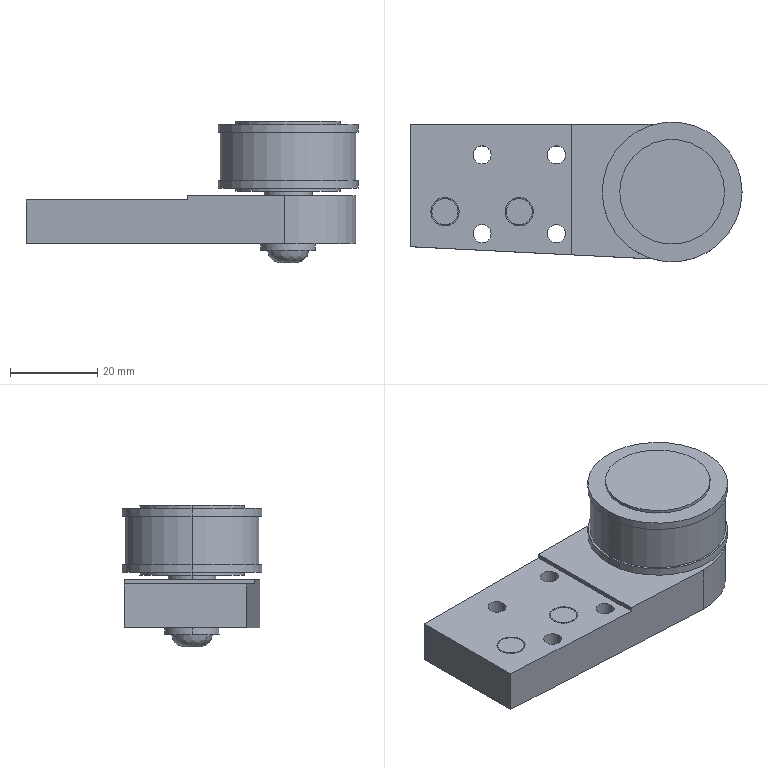Part | STEP file | ASND-0110-Q1-01 | 1 solid | 106 faces | box 76 x 32 x 32.35 mm | volume 32550 mm3 | plane 48 | cylinder 44 | cone 12 | other 2 | commonest cylinder face diameters 4.134 x8 6 x4 6.5 x4 10 x4 12 x4 24 x4